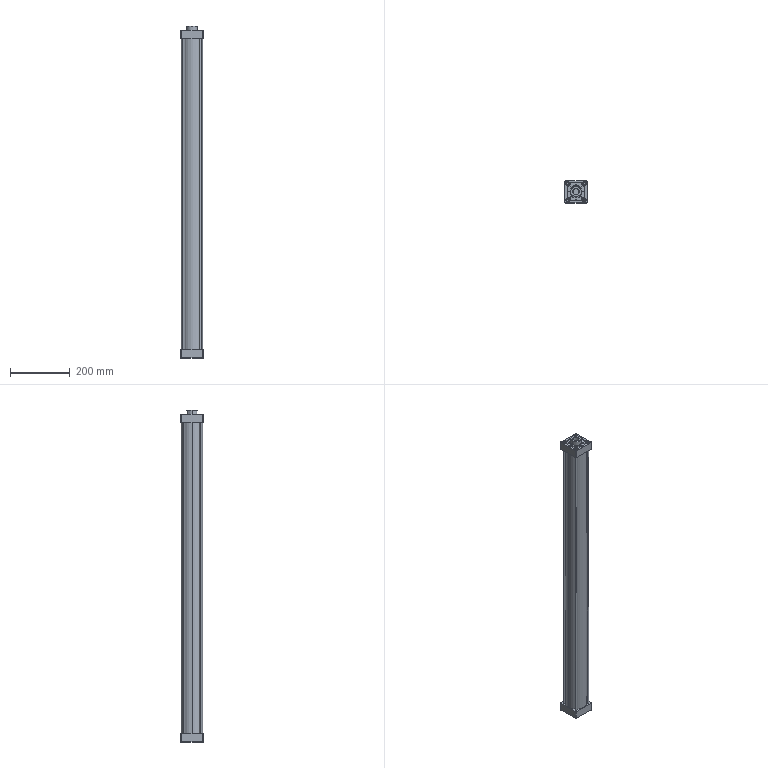Part | SolidWorks | features ICE 10, Fillet 4, Revolution 4, MirrorPattern 3, Chamfer 2, CirPattern 2, Helix 1, RevCut 1, SweepCut 1 | 2 solids | 348 faces | box 75 x 75 x 1111 mm | volume 1290160 mm3 | plane 162 | cylinder 112 | cone 44 | torus 26 | spline 4 | commonest cylinder face diameters 15.806 x30 11.6 x16 12 x16 2 x10 6 x8 8 x8